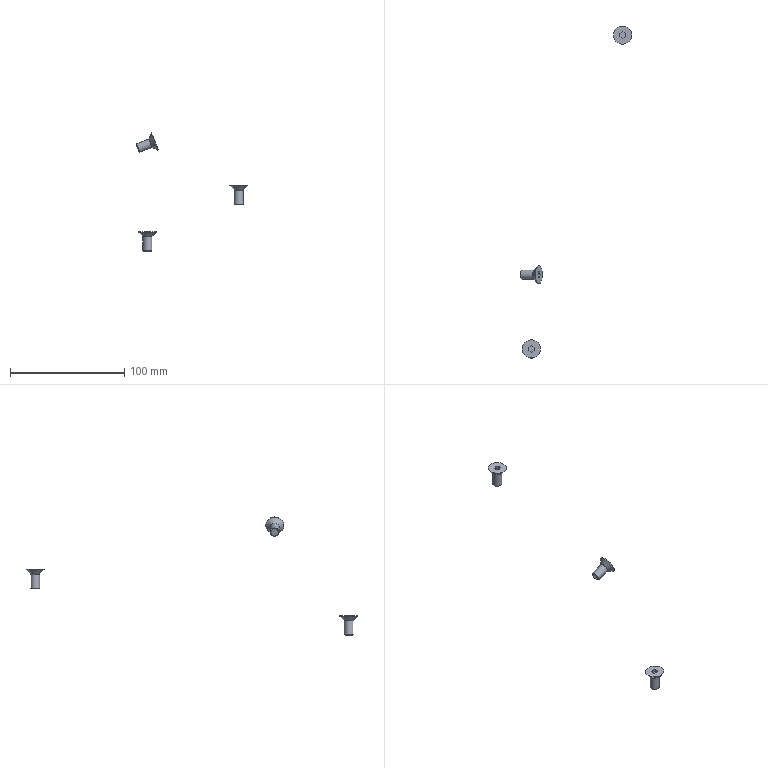Part | STEP file | PTM8.00-20 | 3 solids | 39 faces | box 97.883 x 291 x 103.532 mm | volume 3365 mm3 | plane 27 | cone 6 | cylinder 6 | commonest cylinder face diameters 8 x3 16 x3